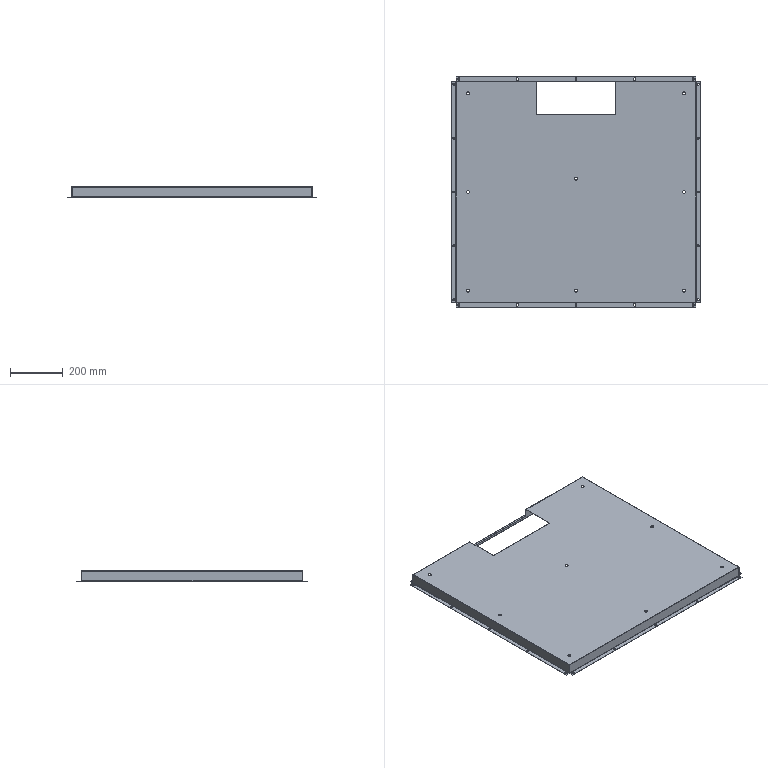Part | 1 solid | 186 faces | box 939 x 869 x 40 mm | volume 898991 mm3 | plane 94 | cylinder 84 | spline 8 | commonest cylinder face diameters 7 x50 11 x16 0.4 x9 2.4 x9